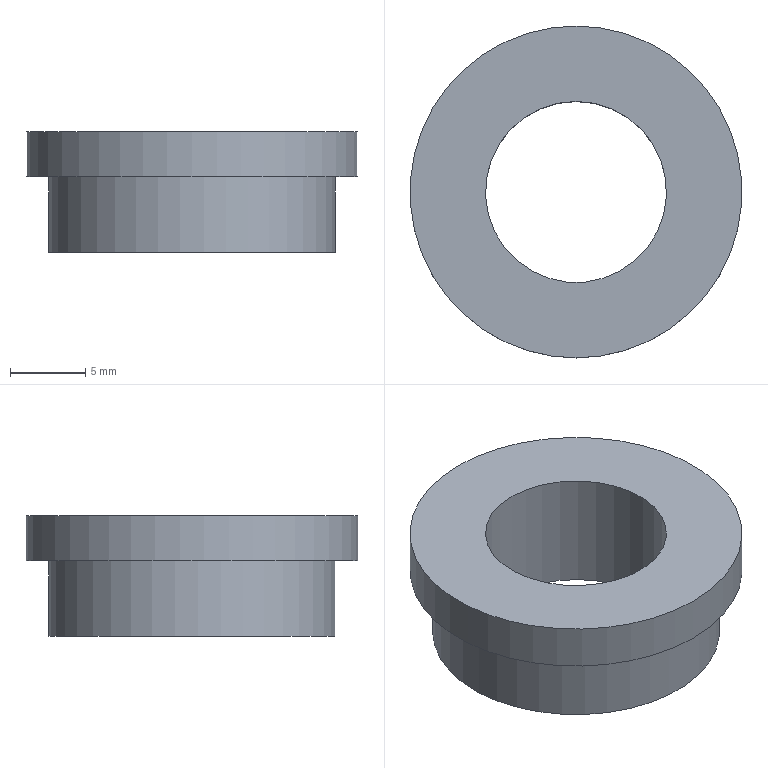Part | STEP file | 1-56.9 | 1 solid | 6 faces | box 22 x 22 x 8 mm | volume 1653 mm3 | plane 3 | cylinder 3 | commonest cylinder face diameters 12 x1 19 x1 22 x1
STEP:
#1=CARTESIAN_POINT('',(0.,0.,0.));
#2=DIRECTION('',(0.,0.,1.));
#3=DIRECTION('',(1.,0.,0.));
#4=AXIS2_PLACEMENT_3D('',#1,#2,#3);
#5=CARTESIAN_POINT('',(0.,9.5,-5.));
#6=VERTEX_POINT('',#5);
#7=CARTESIAN_POINT('',(0.,0.,-5.));
#8=DIRECTION('',(0.,0.,1.));
#9=DIRECTION('',(0.,1.,0.));
#10=AXIS2_PLACEMENT_3D('',#7,#8,#9);
#11=CIRCLE('',#10,9.5);
#12=CARTESIAN_POINT('',(0.,-2.546,-5.));
#13=DIRECTION('',(0.,0.,1.));
#14=DIRECTION('',(1.,0.,0.));
#15=AXIS2_PLACEMENT_3D('',#12,#13,#14);
#16=PLANE('',#15);
#17=CARTESIAN_POINT('',(0.,2.546));
#18=DIRECTION('',(0.,1.));
#19=AXIS2_PLACEMENT_2D('',#17,#18);
#20=CIRCLE('',#19,9.5);
#21=(GEOMETRIC_REPRESENTATION_CONTEXT(2)PARAMETRIC_REPRESENTATION_CONTEXT()REPRESENTATION_CONTEXT('',''));
#22=DEFINITIONAL_REPRESENTATION('',(#20),#21);
#23=PCURVE('',#16,#22);
#24=CARTESIAN_POINT('',(0.,0.,0.));
#25=DIRECTION('',(0.,0.,-1.));
#26=DIRECTION('',(0.,1.,0.));
#27=AXIS2_PLACEMENT_3D('',#24,#25,#26);
#28=CYLINDRICAL_SURFACE('',#27,9.5);
#29=CARTESIAN_POINT('',(6.283,5.));
#30=DIRECTION('',(-1.,0.));
#31=VECTOR('',#30,1.);
#32=LINE('',#29,#31);
#33=(GEOMETRIC_REPRESENTATION_CONTEXT(2)PARAMETRIC_REPRESENTATION_CONTEXT()REPRESENTATION_CONTEXT('',''));
#34=DEFINITIONAL_REPRESENTATION('',(#32),#33);
#35=PCURVE('',#28,#34);
#36=SURFACE_CURVE('',#11,(#23,#35),.PCURVE_S1.);
#37=EDGE_CURVE('',#6,#6,#36,.T.);
#38=ORIENTED_EDGE('',*,*,#37,.T.);
#39=EDGE_LOOP('',(#38));
#40=FACE_BOUND('',#39,.F.);
#41=CARTESIAN_POINT('',(0.,6.,-5.));
#42=VERTEX_POINT('',#41);
#43=CARTESIAN_POINT('',(0.,0.,-5.));
#44=DIRECTION('',(0.,0.,-1.));
#45=DIRECTION('',(0.,1.,0.));
#46=AXIS2_PLACEMENT_3D('',#43,#44,#45);
#47=CIRCLE('',#46,6.);
#48=CARTESIAN_POINT('',(0.,8.546));
#49=CARTESIAN_POINT('',(10.392,8.546));
#50=CARTESIAN_POINT('',(5.196,-0.4545));
#51=CARTESIAN_POINT('',(0.,-9.454));
#52=CARTESIAN_POINT('',(-5.196,-0.4545));
#53=CARTESIAN_POINT('',(-10.392,8.546));
#54=CARTESIAN_POINT('',(0.,8.546));
#55=(BOUNDED_CURVE()B_SPLINE_CURVE(2,(#48,#49,#50,#51,#52,#53,#54),.UNSPECIFIED.,.T.,.F.)B_SPLINE_CURVE_WITH_KNOTS((1,2,2,2,2,1),(-2.094,0.,2.094,4.189,6.283,8.378),.UNSPECIFIED.)CURVE()GEOMETRIC_REPRESENTATION_ITEM()RATIONAL_B_SPLINE_CURVE((1.,0.5,1.,0.5,1.,0.5,1.))REPRESENTATION_ITEM(''));
#56=(GEOMETRIC_REPRESENTATION_CONTEXT(2)PARAMETRIC_REPRESENTATION_CONTEXT()REPRESENTATION_CONTEXT('',''));
#57=DEFINITIONAL_REPRESENTATION('',(#55),#56);
#58=PCURVE('',#16,#57);
#59=CARTESIAN_POINT('',(0.,0.,3.));
#60=DIRECTION('',(0.,0.,-1.));
#61=DIRECTION('',(0.,1.,0.));
#62=AXIS2_PLACEMENT_3D('',#59,#60,#61);
#63=CYLINDRICAL_SURFACE('',#62,6.);
#64=CARTESIAN_POINT('',(0.,8.));
#65=DIRECTION('',(1.,0.));
#66=VECTOR('',#65,1.);
#67=LINE('',#64,#66);
#68=(GEOMETRIC_REPRESENTATION_CONTEXT(2)PARAMETRIC_REPRESENTATION_CONTEXT()REPRESENTATION_CONTEXT('',''));
#69=DEFINITIONAL_REPRESENTATION('',(#67),#68);
#70=PCURVE('',#63,#69);
#71=SURFACE_CURVE('',#47,(#58,#70),.PCURVE_S1.);
#72=EDGE_CURVE('',#42,#42,#71,.T.);
#73=ORIENTED_EDGE('',*,*,#72,.T.);
#74=EDGE_LOOP('',(#73));
#75=FACE_BOUND('',#74,.F.);
#76=ADVANCED_FACE('',(#40,#75),#16,.F.);
#77=CARTESIAN_POINT('',(0.,9.5,0.));
#78=VERTEX_POINT('',#77);
#79=CARTESIAN_POINT('',(0.,9.5,0.));
#80=DIRECTION('',(0.,0.,-1.));
#81=VECTOR('',#80,1.);
#82=LINE('',#79,#81);
#83=CARTESIAN_POINT('',(6.283,0.));
#84=DIRECTION('',(0.,1.));
#85=VECTOR('',#84,1.);
#86=LINE('',#83,#85);
#87=(GEOMETRIC_REPRESENTATION_CONTEXT(2)PARAMETRIC_REPRESENTATION_CONTEXT()REPRESENTATION_CONTEXT('',''));
#88=DEFINITIONAL_REPRESENTATION('',(#86),#87);
#89=PCURVE('',#28,#88);
#90=CARTESIAN_POINT('',(0.,0.));
#91=DIRECTION('',(0.,1.));
#92=VECTOR('',#91,1.);
#93=LINE('',#90,#92);
#94=(GEOMETRIC_REPRESENTATION_CONTEXT(2)PARAMETRIC_REPRESENTATION_CONTEXT()REPRESENTATION_CONTEXT('',''));
#95=DEFINITIONAL_REPRESENTATION('',(#93),#94);
#96=PCURVE('',#28,#95);
#97=SEAM_CURVE('',#82,(#89,#96),.PCURVE_S1.);
#98=EDGE_CURVE('',#78,#6,#97,.T.);
#99=ORIENTED_EDGE('',*,*,#98,.T.);
#100=ORIENTED_EDGE('',*,*,#37,.T.);
#101=ORIENTED_EDGE('',*,*,#98,.F.);
#102=CARTESIAN_POINT('',(0.,0.,0.));
#103=DIRECTION('',(0.,0.,1.));
#104=DIRECTION('',(0.,1.,0.));
#105=AXIS2_PLACEMENT_3D('',#102,#103,#104);
#106=CIRCLE('',#105,9.5);
#107=CARTESIAN_POINT('',(6.283,0.));
#108=DIRECTION('',(-1.,0.));
#109=VECTOR('',#108,1.);
#110=LINE('',#107,#109);
#111=(GEOMETRIC_REPRESENTATION_CONTEXT(2)PARAMETRIC_REPRESENTATION_CONTEXT()REPRESENTATION_CONTEXT('',''));
#112=DEFINITIONAL_REPRESENTATION('',(#110),#111);
#113=PCURVE('',#28,#112);
#114=CARTESIAN_POINT('',(0.,-2.947,0.));
#115=DIRECTION('',(0.,0.,1.));
#116=DIRECTION('',(1.,0.,0.));
#117=AXIS2_PLACEMENT_3D('',#114,#115,#116);
#118=PLANE('',#117);
#119=CARTESIAN_POINT('',(0.,2.947));
#120=DIRECTION('',(0.,1.));
#121=AXIS2_PLACEMENT_2D('',#119,#120);
#122=CIRCLE('',#121,9.5);
#123=(GEOMETRIC_REPRESENTATION_CONTEXT(2)PARAMETRIC_REPRESENTATION_CONTEXT()REPRESENTATION_CONTEXT('',''));
#124=DEFINITIONAL_REPRESENTATION('',(#122),#123);
#125=PCURVE('',#118,#124);
#126=SURFACE_CURVE('',#106,(#113,#125),.PCURVE_S1.);
#127=EDGE_CURVE('',#78,#78,#126,.T.);
#128=ORIENTED_EDGE('',*,*,#127,.F.);
#129=EDGE_LOOP('',(#99,#100,#101,#128));
#130=FACE_BOUND('',#129,.T.);
#131=ADVANCED_FACE('',(#130),#28,.T.);
#132=ORIENTED_EDGE('',*,*,#72,.F.);
#133=CARTESIAN_POINT('',(0.,6.,3.));
#134=VERTEX_POINT('',#133);
#135=CARTESIAN_POINT('',(0.,6.,-5.));
#136=DIRECTION('',(0.,0.,1.));
#137=VECTOR('',#136,1.);
#138=LINE('',#135,#137);
#139=CARTESIAN_POINT('',(0.,8.));
#140=DIRECTION('',(0.,-1.));
#141=VECTOR('',#140,1.);
#142=LINE('',#139,#141);
#143=(GEOMETRIC_REPRESENTATION_CONTEXT(2)PARAMETRIC_REPRESENTATION_CONTEXT()REPRESENTATION_CONTEXT('',''));
#144=DEFINITIONAL_REPRESENTATION('',(#142),#143);
#145=PCURVE('',#63,#144);
#146=CARTESIAN_POINT('',(6.283,8.));
#147=DIRECTION('',(0.,-1.));
#148=VECTOR('',#147,1.);
#149=LINE('',#146,#148);
#150=(GEOMETRIC_REPRESENTATION_CONTEXT(2)PARAMETRIC_REPRESENTATION_CONTEXT()REPRESENTATION_CONTEXT('',''));
#151=DEFINITIONAL_REPRESENTATION('',(#149),#150);
#152=PCURVE('',#63,#151);
#153=SEAM_CURVE('',#138,(#145,#152),.PCURVE_S1.);
#154=EDGE_CURVE('',#42,#134,#153,.T.);
#155=ORIENTED_EDGE('',*,*,#154,.T.);
#156=CARTESIAN_POINT('',(0.,0.,3.));
#157=DIRECTION('',(0.,0.,-1.));
#158=DIRECTION('',(0.,1.,0.));
#159=AXIS2_PLACEMENT_3D('',#156,#157,#158);
#160=CIRCLE('',#159,6.);
#161=CARTESIAN_POINT('',(0.,0.));
#162=DIRECTION('',(1.,0.));
#163=VECTOR('',#162,1.);
#164=LINE('',#161,#163);
#165=(GEOMETRIC_REPRESENTATION_CONTEXT(2)PARAMETRIC_REPRESENTATION_CONTEXT()REPRESENTATION_CONTEXT('',''));
#166=DEFINITIONAL_REPRESENTATION('',(#164),#165);
#167=PCURVE('',#63,#166);
#168=CARTESIAN_POINT('',(0.,-2.947,3.));
#169=DIRECTION('',(0.,0.,1.));
#170=DIRECTION('',(1.,0.,0.));
#171=AXIS2_PLACEMENT_3D('',#168,#169,#170);
#172=PLANE('',#171);
#173=CARTESIAN_POINT('',(0.,8.947));
#174=CARTESIAN_POINT('',(10.392,8.947));
#175=CARTESIAN_POINT('',(5.196,-0.05256));
#176=CARTESIAN_POINT('',(0.,-9.053));
#177=CARTESIAN_POINT('',(-5.196,-0.05256));
#178=CARTESIAN_POINT('',(-10.392,8.947));
#179=CARTESIAN_POINT('',(0.,8.947));
#180=(BOUNDED_CURVE()B_SPLINE_CURVE(2,(#173,#174,#175,#176,#177,#178,#179),.UNSPECIFIED.,.T.,.F.)B_SPLINE_CURVE_WITH_KNOTS((1,2,2,2,2,1),(-2.094,0.,2.094,4.189,6.283,8.378),.UNSPECIFIED.)CURVE()GEOMETRIC_REPRESENTATION_ITEM()RATIONAL_B_SPLINE_CURVE((1.,0.5,1.,0.5,1.,0.5,1.))REPRESENTATION_ITEM(''));
#181=(GEOMETRIC_REPRESENTATION_CONTEXT(2)PARAMETRIC_REPRESENTATION_CONTEXT()REPRESENTATION_CONTEXT('',''));
#182=DEFINITIONAL_REPRESENTATION('',(#180),#181);
#183=PCURVE('',#172,#182);
#184=SURFACE_CURVE('',#160,(#167,#183),.PCURVE_S1.);
#185=EDGE_CURVE('',#134,#134,#184,.T.);
#186=ORIENTED_EDGE('',*,*,#185,.T.);
#187=ORIENTED_EDGE('',*,*,#154,.F.);
#188=EDGE_LOOP('',(#132,#155,#186,#187));
#189=FACE_BOUND('',#188,.F.);
#190=ADVANCED_FACE('',(#189),#63,.F.);
#191=CARTESIAN_POINT('',(0.,11.,0.));
#192=VERTEX_POINT('',#191);
#193=CARTESIAN_POINT('',(0.,0.,0.));
#194=DIRECTION('',(0.,0.,1.));
#195=DIRECTION('',(0.,1.,0.));
#196=AXIS2_PLACEMENT_3D('',#193,#194,#195);
#197=CIRCLE('',#196,11.);
#198=CARTESIAN_POINT('',(0.,2.947));
#199=DIRECTION('',(0.,1.));
#200=AXIS2_PLACEMENT_2D('',#198,#199);
#201=CIRCLE('',#200,11.);
#202=(GEOMETRIC_REPRESENTATION_CONTEXT(2)PARAMETRIC_REPRESENTATION_CONTEXT()REPRESENTATION_CONTEXT('',''));
#203=DEFINITIONAL_REPRESENTATION('',(#201),#202);
#204=PCURVE('',#118,#203);
#205=CARTESIAN_POINT('',(0.,0.,0.));
#206=DIRECTION('',(0.,0.,1.));
#207=DIRECTION('',(0.,1.,0.));
#208=AXIS2_PLACEMENT_3D('',#205,#206,#207);
#209=CYLINDRICAL_SURFACE('',#208,11.);
#210=CARTESIAN_POINT('',(0.,0.));
#211=DIRECTION('',(1.,0.));
#212=VECTOR('',#211,1.);
#213=LINE('',#210,#212);
#214=(GEOMETRIC_REPRESENTATION_CONTEXT(2)PARAMETRIC_REPRESENTATION_CONTEXT()REPRESENTATION_CONTEXT('',''));
#215=DEFINITIONAL_REPRESENTATION('',(#213),#214);
#216=PCURVE('',#209,#215);
#217=SURFACE_CURVE('',#197,(#204,#216),.PCURVE_S1.);
#218=EDGE_CURVE('',#192,#192,#217,.T.);
#219=ORIENTED_EDGE('',*,*,#218,.T.);
#220=EDGE_LOOP('',(#219));
#221=FACE_BOUND('',#220,.F.);
#222=ORIENTED_EDGE('',*,*,#127,.F.);
#223=EDGE_LOOP('',(#222));
#224=FACE_BOUND('',#223,.F.);
#225=ADVANCED_FACE('',(#221,#224),#118,.F.);
#226=ORIENTED_EDGE('',*,*,#218,.T.);
#227=CARTESIAN_POINT('',(0.,11.,3.));
#228=VERTEX_POINT('',#227);
#229=CARTESIAN_POINT('',(0.,11.,0.));
#230=DIRECTION('',(0.,0.,1.));
#231=VECTOR('',#230,1.);
#232=LINE('',#229,#231);
#233=CARTESIAN_POINT('',(6.283,0.));
#234=DIRECTION('',(0.,1.));
#235=VECTOR('',#234,1.);
#236=LINE('',#233,#235);
#237=(GEOMETRIC_REPRESENTATION_CONTEXT(2)PARAMETRIC_REPRESENTATION_CONTEXT()REPRESENTATION_CONTEXT('',''));
#238=DEFINITIONAL_REPRESENTATION('',(#236),#237);
#239=PCURVE('',#209,#238);
#240=CARTESIAN_POINT('',(0.,0.));
#241=DIRECTION('',(0.,1.));
#242=VECTOR('',#241,1.);
#243=LINE('',#240,#242);
#244=(GEOMETRIC_REPRESENTATION_CONTEXT(2)PARAMETRIC_REPRESENTATION_CONTEXT()REPRESENTATION_CONTEXT('',''));
#245=DEFINITIONAL_REPRESENTATION('',(#243),#244);
#246=PCURVE('',#209,#245);
#247=SEAM_CURVE('',#232,(#239,#246),.PCURVE_S1.);
#248=EDGE_CURVE('',#192,#228,#247,.T.);
#249=ORIENTED_EDGE('',*,*,#248,.T.);
#250=CARTESIAN_POINT('',(0.,0.,3.));
#251=DIRECTION('',(0.,0.,1.));
#252=DIRECTION('',(0.,1.,0.));
#253=AXIS2_PLACEMENT_3D('',#250,#251,#252);
#254=CIRCLE('',#253,11.);
#255=CARTESIAN_POINT('',(0.,3.));
#256=DIRECTION('',(1.,0.));
#257=VECTOR('',#256,1.);
#258=LINE('',#255,#257);
#259=(GEOMETRIC_REPRESENTATION_CONTEXT(2)PARAMETRIC_REPRESENTATION_CONTEXT()REPRESENTATION_CONTEXT('',''));
#260=DEFINITIONAL_REPRESENTATION('',(#258),#259);
#261=PCURVE('',#209,#260);
#262=CARTESIAN_POINT('',(0.,2.947));
#263=DIRECTION('',(0.,1.));
#264=AXIS2_PLACEMENT_2D('',#262,#263);
#265=CIRCLE('',#264,11.);
#266=(GEOMETRIC_REPRESENTATION_CONTEXT(2)PARAMETRIC_REPRESENTATION_CONTEXT()REPRESENTATION_CONTEXT('',''));
#267=DEFINITIONAL_REPRESENTATION('',(#265),#266);
#268=PCURVE('',#172,#267);
#269=SURFACE_CURVE('',#254,(#261,#268),.PCURVE_S1.);
#270=EDGE_CURVE('',#228,#228,#269,.T.);
#271=ORIENTED_EDGE('',*,*,#270,.F.);
#272=ORIENTED_EDGE('',*,*,#248,.F.);
#273=EDGE_LOOP('',(#226,#249,#271,#272));
#274=FACE_BOUND('',#273,.T.);
#275=ADVANCED_FACE('',(#274),#209,.T.);
#276=ORIENTED_EDGE('',*,*,#270,.T.);
#277=EDGE_LOOP('',(#276));
#278=FACE_BOUND('',#277,.T.);
#279=ORIENTED_EDGE('',*,*,#185,.T.);
#280=EDGE_LOOP('',(#279));
#281=FACE_BOUND('',#280,.T.);
#282=ADVANCED_FACE('',(#278,#281),#172,.T.);
#283=CLOSED_SHELL('',(#76,#131,#190,#225,#275,#282));
#284=MANIFOLD_SOLID_BREP('',#283);
#285=(LENGTH_UNIT()NAMED_UNIT(*)SI_UNIT(.MILLI.,.METRE.));
#286=UNCERTAINTY_MEASURE_WITH_UNIT(LENGTH_MEASURE(0.0000001),#285,'','');
#287=(NAMED_UNIT(*)PLANE_ANGLE_UNIT()SI_UNIT($,.RADIAN.));
#288=(NAMED_UNIT(*)SI_UNIT($,.STERADIAN.)SOLID_ANGLE_UNIT());
#289=(GEOMETRIC_REPRESENTATION_CONTEXT(3)GLOBAL_UNCERTAINTY_ASSIGNED_CONTEXT((#286))GLOBAL_UNIT_ASSIGNED_CONTEXT((#285,#287,#288))REPRESENTATION_CONTEXT('',''));
#290=ADVANCED_BREP_SHAPE_REPRESENTATION('',(#4,#284),#289);